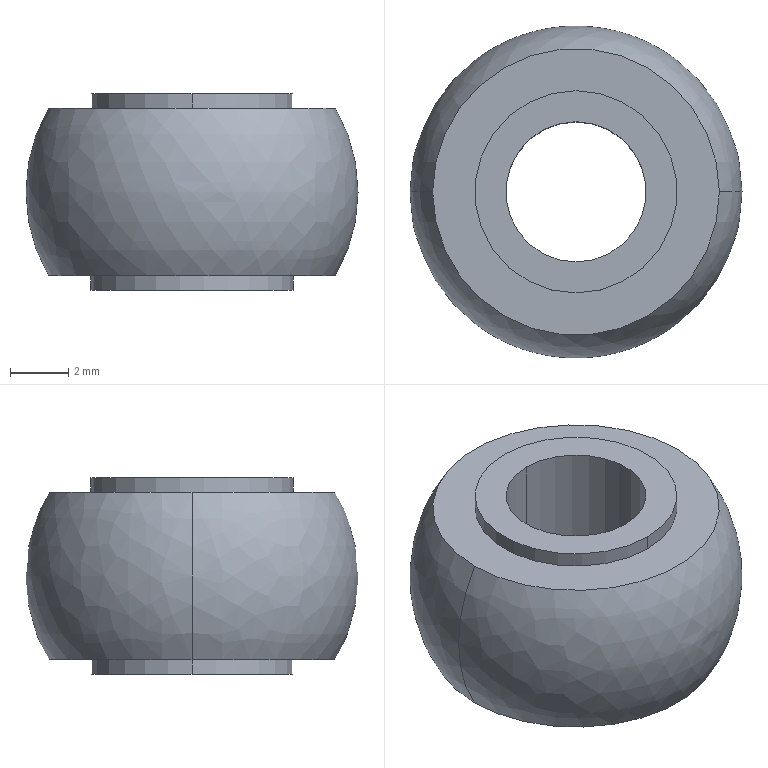Part | SolidWorks | features BaseBody 1 | 1 solid | 12 faces | box 11.43 x 11.396 x 6.782 mm | volume 456.05 mm3 | cylinder 6 | plane 4 | spline 2 | commonest cylinder face diameters 6.961 x4 4.826 x2
STEP:
#1=CARTESIAN_POINT('',(4.935,0.,2.883));
#2=VERTEX_POINT('',#1);
#3=CARTESIAN_POINT('',(-4.935,0.,2.883));
#4=VERTEX_POINT('',#3);
#5=CARTESIAN_POINT('',(0.,0.,2.883));
#6=DIRECTION('',(0.,0.,1.));
#7=DIRECTION('',(-1.,0.,0.));
#8=AXIS2_PLACEMENT_3D('',#5,#6,#7);
#9=CIRCLE('',#8,4.935);
#10=EDGE_CURVE('',#2,#4,#9,.T.);
#11=ORIENTED_EDGE('',*,*,#10,.F.);
#12=CARTESIAN_POINT('',(4.935,0.,-2.883));
#13=VERTEX_POINT('',#12);
#14=CARTESIAN_POINT('',(0.,0.,0.));
#15=DIRECTION('',(0.,1.,0.));
#16=DIRECTION('',(0.,0.,1.));
#17=AXIS2_PLACEMENT_3D('',#14,#15,#16);
#18=CIRCLE('',#17,5.715);
#19=EDGE_CURVE('',#2,#13,#18,.T.);
#20=ORIENTED_EDGE('',*,*,#19,.T.);
#21=CARTESIAN_POINT('',(-4.935,0.,-2.883));
#22=VERTEX_POINT('',#21);
#23=CARTESIAN_POINT('',(0.,0.,-2.883));
#24=DIRECTION('',(0.,0.,-1.));
#25=DIRECTION('',(-1.,0.,0.));
#26=AXIS2_PLACEMENT_3D('',#23,#24,#25);
#27=CIRCLE('',#26,4.935);
#28=EDGE_CURVE('',#22,#13,#27,.T.);
#29=ORIENTED_EDGE('',*,*,#28,.F.);
#30=CARTESIAN_POINT('',(0.,0.,0.));
#31=DIRECTION('',(0.,-1.,0.));
#32=DIRECTION('',(0.,0.,1.));
#33=AXIS2_PLACEMENT_3D('',#30,#31,#32);
#34=CIRCLE('',#33,5.715);
#35=EDGE_CURVE('',#4,#22,#34,.T.);
#36=ORIENTED_EDGE('',*,*,#35,.F.);
#37=EDGE_LOOP('',(#11,#20,#29,#36));
#38=FACE_OUTER_BOUND('',#37,.T.);
#39=CARTESIAN_POINT('',(-4.935,0.,2.883));
#40=CARTESIAN_POINT('',(-4.935,9.869,2.883));
#41=CARTESIAN_POINT('',(4.935,9.869,2.883));
#42=CARTESIAN_POINT('',(4.935,0.,2.883));
#43=CARTESIAN_POINT('',(-6.001,0.,1.057));
#44=CARTESIAN_POINT('',(-6.001,12.002,1.057));
#45=CARTESIAN_POINT('',(6.001,12.002,1.057));
#46=CARTESIAN_POINT('',(6.001,0.,1.057));
#47=CARTESIAN_POINT('',(-6.001,0.,-1.057));
#48=CARTESIAN_POINT('',(-6.001,12.002,-1.057));
#49=CARTESIAN_POINT('',(6.001,12.002,-1.057));
#50=CARTESIAN_POINT('',(6.001,0.,-1.057));
#51=CARTESIAN_POINT('',(-4.935,0.,-2.883));
#52=CARTESIAN_POINT('',(-4.935,9.869,-2.883));
#53=CARTESIAN_POINT('',(4.935,9.869,-2.883));
#54=CARTESIAN_POINT('',(4.935,0.,-2.883));
#55=(BOUNDED_SURFACE()B_SPLINE_SURFACE(3,3,((#39,#40,#41,#42),(#43,#44,#45,#46),(#47,#48,#49,#50),(#51,#52,#53,#54)),.UNSPECIFIED.,.F.,.F.,.F.)B_SPLINE_SURFACE_WITH_KNOTS((4,4),(4,4),(0.,1.),(0.,1.),.UNSPECIFIED.)GEOMETRIC_REPRESENTATION_ITEM()RATIONAL_B_SPLINE_SURFACE(((1.,0.3333,0.3333,1.),(0.909,0.303,0.303,0.909),(0.909,0.303,0.303,0.909),(1.,0.3333,0.3333,1.)))REPRESENTATION_ITEM('')SURFACE());
#56=ADVANCED_FACE('',(#38),#55,.F.);
#57=CARTESIAN_POINT('',(0.,2.413,3.391));
#58=VERTEX_POINT('',#57);
#59=CARTESIAN_POINT('',(0.,-2.413,3.391));
#60=VERTEX_POINT('',#59);
#61=CARTESIAN_POINT('',(0.,0.,3.391));
#62=DIRECTION('',(0.,0.,1.));
#63=DIRECTION('',(0.,1.,0.));
#64=AXIS2_PLACEMENT_3D('',#61,#62,#63);
#65=CIRCLE('',#64,2.413);
#66=EDGE_CURVE('',#58,#60,#65,.T.);
#67=ORIENTED_EDGE('',*,*,#66,.T.);
#68=CARTESIAN_POINT('',(0.,-2.413,-3.391));
#69=VERTEX_POINT('',#68);
#70=CARTESIAN_POINT('',(0.,-2.413,3.391));
#71=DIRECTION('',(0.,0.,-1.));
#72=VECTOR('',#71,1000.);
#73=LINE('',#70,#72);
#74=EDGE_CURVE('',#60,#69,#73,.T.);
#75=ORIENTED_EDGE('',*,*,#74,.T.);
#76=CARTESIAN_POINT('',(0.,2.413,-3.391));
#77=VERTEX_POINT('',#76);
#78=CARTESIAN_POINT('',(0.,0.,-3.391));
#79=DIRECTION('',(0.,0.,-1.));
#80=DIRECTION('',(0.,1.,0.));
#81=AXIS2_PLACEMENT_3D('',#78,#79,#80);
#82=CIRCLE('',#81,2.413);
#83=EDGE_CURVE('',#69,#77,#82,.T.);
#84=ORIENTED_EDGE('',*,*,#83,.T.);
#85=CARTESIAN_POINT('',(0.,2.413,3.391));
#86=DIRECTION('',(0.,0.,-1.));
#87=VECTOR('',#86,1000.);
#88=LINE('',#85,#87);
#89=EDGE_CURVE('',#58,#77,#88,.T.);
#90=ORIENTED_EDGE('',*,*,#89,.F.);
#91=EDGE_LOOP('',(#67,#75,#84,#90));
#92=FACE_OUTER_BOUND('',#91,.T.);
#93=CARTESIAN_POINT('',(0.,0.,3.391));
#94=DIRECTION('',(0.,0.,-1.));
#95=DIRECTION('',(0.,1.,0.));
#96=AXIS2_PLACEMENT_3D('',#93,#94,#95);
#97=CYLINDRICAL_SURFACE('',#96,2.413);
#98=ADVANCED_FACE('',(#92),#97,.F.);
#99=CARTESIAN_POINT('',(3.481,0.,-2.883));
#100=VERTEX_POINT('',#99);
#101=CARTESIAN_POINT('',(-3.481,0.,-2.883));
#102=VERTEX_POINT('',#101);
#103=CARTESIAN_POINT('',(0.,0.,-2.883));
#104=DIRECTION('',(0.,0.,1.));
#105=DIRECTION('',(-1.,0.,0.));
#106=AXIS2_PLACEMENT_3D('',#103,#104,#105);
#107=CIRCLE('',#106,3.481);
#108=EDGE_CURVE('',#100,#102,#107,.T.);
#109=ORIENTED_EDGE('',*,*,#108,.F.);
#110=CARTESIAN_POINT('',(3.481,0.,-3.391));
#111=VERTEX_POINT('',#110);
#112=CARTESIAN_POINT('',(3.481,0.,-2.883));
#113=DIRECTION('',(0.,0.,-1.));
#114=VECTOR('',#113,1000.);
#115=LINE('',#112,#114);
#116=EDGE_CURVE('',#100,#111,#115,.T.);
#117=ORIENTED_EDGE('',*,*,#116,.T.);
#118=CARTESIAN_POINT('',(-3.481,0.,-3.391));
#119=VERTEX_POINT('',#118);
#120=CARTESIAN_POINT('',(0.,0.,-3.391));
#121=DIRECTION('',(0.,0.,-1.));
#122=DIRECTION('',(-1.,0.,0.));
#123=AXIS2_PLACEMENT_3D('',#120,#121,#122);
#124=CIRCLE('',#123,3.481);
#125=EDGE_CURVE('',#119,#111,#124,.T.);
#126=ORIENTED_EDGE('',*,*,#125,.F.);
#127=CARTESIAN_POINT('',(-3.481,0.,-2.883));
#128=DIRECTION('',(0.,0.,-1.));
#129=VECTOR('',#128,1000.);
#130=LINE('',#127,#129);
#131=EDGE_CURVE('',#102,#119,#130,.T.);
#132=ORIENTED_EDGE('',*,*,#131,.F.);
#133=EDGE_LOOP('',(#109,#117,#126,#132));
#134=FACE_OUTER_BOUND('',#133,.T.);
#135=CARTESIAN_POINT('',(0.,0.,-2.883));
#136=DIRECTION('',(0.,0.,-1.));
#137=DIRECTION('',(-1.,0.,0.));
#138=AXIS2_PLACEMENT_3D('',#135,#136,#137);
#139=CYLINDRICAL_SURFACE('',#138,3.481);
#140=ADVANCED_FACE('',(#134),#139,.T.);
#141=CARTESIAN_POINT('',(0.,-3.481,3.391));
#142=VERTEX_POINT('',#141);
#143=CARTESIAN_POINT('',(0.,3.481,3.391));
#144=VERTEX_POINT('',#143);
#145=CARTESIAN_POINT('',(0.,0.,3.391));
#146=DIRECTION('',(0.,0.,1.));
#147=DIRECTION('',(0.,1.,0.));
#148=AXIS2_PLACEMENT_3D('',#145,#146,#147);
#149=CIRCLE('',#148,3.481);
#150=EDGE_CURVE('',#142,#144,#149,.T.);
#151=ORIENTED_EDGE('',*,*,#150,.F.);
#152=CARTESIAN_POINT('',(0.,-3.481,2.883));
#153=VERTEX_POINT('',#152);
#154=CARTESIAN_POINT('',(0.,-3.481,3.391));
#155=DIRECTION('',(0.,0.,-1.));
#156=VECTOR('',#155,1000.);
#157=LINE('',#154,#156);
#158=EDGE_CURVE('',#142,#153,#157,.T.);
#159=ORIENTED_EDGE('',*,*,#158,.T.);
#160=CARTESIAN_POINT('',(0.,3.481,2.883));
#161=VERTEX_POINT('',#160);
#162=CARTESIAN_POINT('',(0.,0.,2.883));
#163=DIRECTION('',(0.,0.,-1.));
#164=DIRECTION('',(0.,1.,0.));
#165=AXIS2_PLACEMENT_3D('',#162,#163,#164);
#166=CIRCLE('',#165,3.481);
#167=EDGE_CURVE('',#161,#153,#166,.T.);
#168=ORIENTED_EDGE('',*,*,#167,.F.);
#169=CARTESIAN_POINT('',(0.,3.481,3.391));
#170=DIRECTION('',(0.,0.,-1.));
#171=VECTOR('',#170,1000.);
#172=LINE('',#169,#171);
#173=EDGE_CURVE('',#144,#161,#172,.T.);
#174=ORIENTED_EDGE('',*,*,#173,.F.);
#175=EDGE_LOOP('',(#151,#159,#168,#174));
#176=FACE_OUTER_BOUND('',#175,.T.);
#177=CARTESIAN_POINT('',(0.,0.,3.391));
#178=DIRECTION('',(0.,0.,-1.));
#179=DIRECTION('',(0.,1.,0.));
#180=AXIS2_PLACEMENT_3D('',#177,#178,#179);
#181=CYLINDRICAL_SURFACE('',#180,3.481);
#182=ADVANCED_FACE('',(#176),#181,.T.);
#183=ORIENTED_EDGE('',*,*,#74,.F.);
#184=CARTESIAN_POINT('',(0.,0.,3.391));
#185=DIRECTION('',(0.,0.,1.));
#186=DIRECTION('',(0.,1.,0.));
#187=AXIS2_PLACEMENT_3D('',#184,#185,#186);
#188=CIRCLE('',#187,2.413);
#189=EDGE_CURVE('',#60,#58,#188,.T.);
#190=ORIENTED_EDGE('',*,*,#189,.T.);
#191=ORIENTED_EDGE('',*,*,#89,.T.);
#192=CARTESIAN_POINT('',(0.,0.,-3.391));
#193=DIRECTION('',(0.,0.,-1.));
#194=DIRECTION('',(0.,1.,0.));
#195=AXIS2_PLACEMENT_3D('',#192,#193,#194);
#196=CIRCLE('',#195,2.413);
#197=EDGE_CURVE('',#77,#69,#196,.T.);
#198=ORIENTED_EDGE('',*,*,#197,.T.);
#199=EDGE_LOOP('',(#183,#190,#191,#198));
#200=FACE_OUTER_BOUND('',#199,.T.);
#201=CARTESIAN_POINT('',(0.,0.,3.391));
#202=DIRECTION('',(0.,0.,-1.));
#203=DIRECTION('',(0.,1.,0.));
#204=AXIS2_PLACEMENT_3D('',#201,#202,#203);
#205=CYLINDRICAL_SURFACE('',#204,2.413);
#206=ADVANCED_FACE('',(#200),#205,.F.);
#207=ORIENTED_EDGE('',*,*,#197,.F.);
#208=ORIENTED_EDGE('',*,*,#83,.F.);
#209=EDGE_LOOP('',(#207,#208));
#210=FACE_BOUND('',#209,.T.);
#211=ORIENTED_EDGE('',*,*,#125,.T.);
#212=CARTESIAN_POINT('',(0.,0.,-3.391));
#213=DIRECTION('',(0.,0.,-1.));
#214=DIRECTION('',(-1.,0.,0.));
#215=AXIS2_PLACEMENT_3D('',#212,#213,#214);
#216=CIRCLE('',#215,3.481);
#217=EDGE_CURVE('',#111,#119,#216,.T.);
#218=ORIENTED_EDGE('',*,*,#217,.T.);
#219=EDGE_LOOP('',(#211,#218));
#220=FACE_OUTER_BOUND('',#219,.T.);
#221=CARTESIAN_POINT('',(3.522,-3.522,-3.391));
#222=DIRECTION('',(0.,0.,-1.));
#223=DIRECTION('',(-1.,0.,0.));
#224=AXIS2_PLACEMENT_3D('',#221,#222,#223);
#225=PLANE('',#224);
#226=ADVANCED_FACE('',(#210,#220),#225,.T.);
#227=ORIENTED_EDGE('',*,*,#66,.F.);
#228=ORIENTED_EDGE('',*,*,#189,.F.);
#229=EDGE_LOOP('',(#227,#228));
#230=FACE_BOUND('',#229,.T.);
#231=CARTESIAN_POINT('',(0.,0.,3.391));
#232=DIRECTION('',(0.,0.,1.));
#233=DIRECTION('',(0.,1.,0.));
#234=AXIS2_PLACEMENT_3D('',#231,#232,#233);
#235=CIRCLE('',#234,3.481);
#236=EDGE_CURVE('',#144,#142,#235,.T.);
#237=ORIENTED_EDGE('',*,*,#236,.T.);
#238=ORIENTED_EDGE('',*,*,#150,.T.);
#239=EDGE_LOOP('',(#237,#238));
#240=FACE_OUTER_BOUND('',#239,.T.);
#241=CARTESIAN_POINT('',(-3.522,-3.522,3.391));
#242=DIRECTION('',(0.,0.,1.));
#243=DIRECTION('',(1.,0.,0.));
#244=AXIS2_PLACEMENT_3D('',#241,#242,#243);
#245=PLANE('',#244);
#246=ADVANCED_FACE('',(#230,#240),#245,.T.);
#247=ORIENTED_EDGE('',*,*,#116,.F.);
#248=CARTESIAN_POINT('',(0.,0.,-2.883));
#249=DIRECTION('',(0.,0.,1.));
#250=DIRECTION('',(-1.,0.,0.));
#251=AXIS2_PLACEMENT_3D('',#248,#249,#250);
#252=CIRCLE('',#251,3.481);
#253=EDGE_CURVE('',#102,#100,#252,.T.);
#254=ORIENTED_EDGE('',*,*,#253,.F.);
#255=ORIENTED_EDGE('',*,*,#131,.T.);
#256=ORIENTED_EDGE('',*,*,#217,.F.);
#257=EDGE_LOOP('',(#247,#254,#255,#256));
#258=FACE_OUTER_BOUND('',#257,.T.);
#259=CARTESIAN_POINT('',(0.,0.,-2.883));
#260=DIRECTION('',(0.,0.,-1.));
#261=DIRECTION('',(-1.,0.,0.));
#262=AXIS2_PLACEMENT_3D('',#259,#260,#261);
#263=CYLINDRICAL_SURFACE('',#262,3.481);
#264=ADVANCED_FACE('',(#258),#263,.T.);
#265=ORIENTED_EDGE('',*,*,#158,.F.);
#266=ORIENTED_EDGE('',*,*,#236,.F.);
#267=ORIENTED_EDGE('',*,*,#173,.T.);
#268=CARTESIAN_POINT('',(0.,0.,2.883));
#269=DIRECTION('',(0.,0.,-1.));
#270=DIRECTION('',(0.,1.,0.));
#271=AXIS2_PLACEMENT_3D('',#268,#269,#270);
#272=CIRCLE('',#271,3.481);
#273=EDGE_CURVE('',#153,#161,#272,.T.);
#274=ORIENTED_EDGE('',*,*,#273,.F.);
#275=EDGE_LOOP('',(#265,#266,#267,#274));
#276=FACE_OUTER_BOUND('',#275,.T.);
#277=CARTESIAN_POINT('',(0.,0.,3.391));
#278=DIRECTION('',(0.,0.,-1.));
#279=DIRECTION('',(0.,1.,0.));
#280=AXIS2_PLACEMENT_3D('',#277,#278,#279);
#281=CYLINDRICAL_SURFACE('',#280,3.481);
#282=ADVANCED_FACE('',(#276),#281,.T.);
#283=ORIENTED_EDGE('',*,*,#253,.T.);
#284=ORIENTED_EDGE('',*,*,#108,.T.);
#285=EDGE_LOOP('',(#283,#284));
#286=FACE_BOUND('',#285,.T.);
#287=ORIENTED_EDGE('',*,*,#28,.T.);
#288=CARTESIAN_POINT('',(0.,0.,-2.883));
#289=DIRECTION('',(0.,0.,-1.));
#290=DIRECTION('',(-1.,0.,0.));
#291=AXIS2_PLACEMENT_3D('',#288,#289,#290);
#292=CIRCLE('',#291,4.935);
#293=EDGE_CURVE('',#13,#22,#292,.T.);
#294=ORIENTED_EDGE('',*,*,#293,.T.);
#295=EDGE_LOOP('',(#287,#294));
#296=FACE_OUTER_BOUND('',#295,.T.);
#297=CARTESIAN_POINT('',(4.994,-4.994,-2.883));
#298=DIRECTION('',(0.,0.,-1.));
#299=DIRECTION('',(-1.,0.,0.));
#300=AXIS2_PLACEMENT_3D('',#297,#298,#299);
#301=PLANE('',#300);
#302=ADVANCED_FACE('',(#286,#296),#301,.T.);
#303=ORIENTED_EDGE('',*,*,#167,.T.);
#304=ORIENTED_EDGE('',*,*,#273,.T.);
#305=EDGE_LOOP('',(#303,#304));
#306=FACE_BOUND('',#305,.T.);
#307=CARTESIAN_POINT('',(0.,0.,2.883));
#308=DIRECTION('',(0.,0.,1.));
#309=DIRECTION('',(-1.,0.,0.));
#310=AXIS2_PLACEMENT_3D('',#307,#308,#309);
#311=CIRCLE('',#310,4.935);
#312=EDGE_CURVE('',#4,#2,#311,.T.);
#313=ORIENTED_EDGE('',*,*,#312,.T.);
#314=ORIENTED_EDGE('',*,*,#10,.T.);
#315=EDGE_LOOP('',(#313,#314));
#316=FACE_OUTER_BOUND('',#315,.T.);
#317=CARTESIAN_POINT('',(-4.994,-4.994,2.883));
#318=DIRECTION('',(0.,0.,1.));
#319=DIRECTION('',(1.,0.,0.));
#320=AXIS2_PLACEMENT_3D('',#317,#318,#319);
#321=PLANE('',#320);
#322=ADVANCED_FACE('',(#306,#316),#321,.T.);
#323=ORIENTED_EDGE('',*,*,#19,.F.);
#324=ORIENTED_EDGE('',*,*,#312,.F.);
#325=ORIENTED_EDGE('',*,*,#35,.T.);
#326=ORIENTED_EDGE('',*,*,#293,.F.);
#327=EDGE_LOOP('',(#323,#324,#325,#326));
#328=FACE_OUTER_BOUND('',#327,.T.);
#329=CARTESIAN_POINT('',(4.935,0.,2.883));
#330=CARTESIAN_POINT('',(4.935,-9.869,2.883));
#331=CARTESIAN_POINT('',(-4.935,-9.869,2.883));
#332=CARTESIAN_POINT('',(-4.935,0.,2.883));
#333=CARTESIAN_POINT('',(6.001,0.,1.057));
#334=CARTESIAN_POINT('',(6.001,-12.002,1.057));
#335=CARTESIAN_POINT('',(-6.001,-12.002,1.057));
#336=CARTESIAN_POINT('',(-6.001,0.,1.057));
#337=CARTESIAN_POINT('',(6.001,0.,-1.057));
#338=CARTESIAN_POINT('',(6.001,-12.002,-1.057));
#339=CARTESIAN_POINT('',(-6.001,-12.002,-1.057));
#340=CARTESIAN_POINT('',(-6.001,0.,-1.057));
#341=CARTESIAN_POINT('',(4.935,0.,-2.883));
#342=CARTESIAN_POINT('',(4.935,-9.869,-2.883));
#343=CARTESIAN_POINT('',(-4.935,-9.869,-2.883));
#344=CARTESIAN_POINT('',(-4.935,0.,-2.883));
#345=(BOUNDED_SURFACE()B_SPLINE_SURFACE(3,3,((#329,#330,#331,#332),(#333,#334,#335,#336),(#337,#338,#339,#340),(#341,#342,#343,#344)),.UNSPECIFIED.,.F.,.F.,.F.)B_SPLINE_SURFACE_WITH_KNOTS((4,4),(4,4),(0.,1.),(0.,1.),.UNSPECIFIED.)GEOMETRIC_REPRESENTATION_ITEM()RATIONAL_B_SPLINE_SURFACE(((1.,0.3333,0.3333,1.),(0.909,0.303,0.303,0.909),(0.909,0.303,0.303,0.909),(1.,0.3333,0.3333,1.)))REPRESENTATION_ITEM('')SURFACE());
#346=ADVANCED_FACE('',(#328),#345,.F.);
#347=CLOSED_SHELL('',(#56,#98,#140,#182,#206,#226,#246,#264,#282,#302,#322,#346));
#348=MANIFOLD_SOLID_BREP('',#347);
#349=CARTESIAN_POINT('',(0.,0.,0.));
#350=DIRECTION('',(0.,0.,1.));
#351=DIRECTION('',(1.,0.,0.));
#352=AXIS2_PLACEMENT_3D('',#349,#350,#351);
#353=(LENGTH_UNIT()NAMED_UNIT(*)SI_UNIT(.MILLI.,.METRE.));
#354=UNCERTAINTY_MEASURE_WITH_UNIT(LENGTH_MEASURE(0.00001),#353,'','');
#355=(NAMED_UNIT(*)PLANE_ANGLE_UNIT()SI_UNIT($,.RADIAN.));
#356=(NAMED_UNIT(*)SI_UNIT($,.STERADIAN.)SOLID_ANGLE_UNIT());
#357=(GEOMETRIC_REPRESENTATION_CONTEXT(3)GLOBAL_UNCERTAINTY_ASSIGNED_CONTEXT((#354))GLOBAL_UNIT_ASSIGNED_CONTEXT((#353,#355,#356))REPRESENTATION_CONTEXT('',''));
#358=ADVANCED_BREP_SHAPE_REPRESENTATION('',(#348,#352),#357);